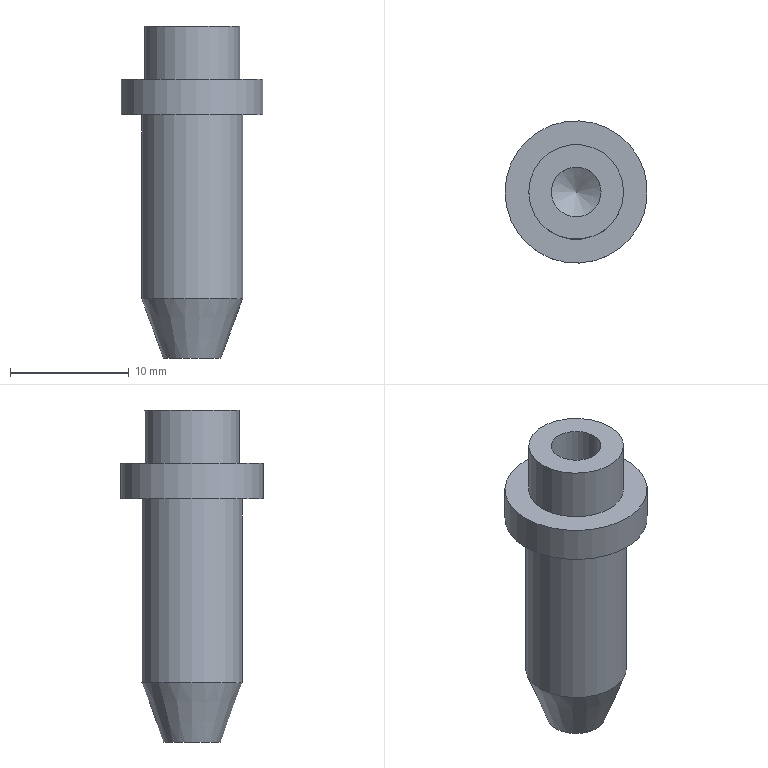Part | NX | features BREP 1 | 1 solid | 10 faces | box 12 x 12 x 28 mm | volume 1447 mm3 | plane 4 | cylinder 4 | cone 2 | commonest cylinder face diameters 4.2 x1 8 x1 8.5 x1 12 x1
STEP:
#1=CARTESIAN_POINT('',(2.1,0.,0.));
#2=VERTEX_POINT('',#1);
#3=CARTESIAN_POINT('',(0.,0.,0.));
#4=DIRECTION('',(0.,0.,1.));
#5=DIRECTION('',(1.,0.,0.));
#6=AXIS2_PLACEMENT_3D('',#3,#4,#5);
#7=CIRCLE('',#6,2.1);
#8=EDGE_CURVE('',#2,#2,#7,.T.);
#9=ORIENTED_EDGE('',*,*,#8,.F.);
#10=EDGE_LOOP('',(#9));
#11=FACE_BOUND('',#10,.T.);
#12=CARTESIAN_POINT('',(-4.,0.,0.));
#13=VERTEX_POINT('',#12);
#14=CARTESIAN_POINT('',(0.,0.,0.));
#15=DIRECTION('',(0.,0.,-1.));
#16=DIRECTION('',(-1.,0.,0.));
#17=AXIS2_PLACEMENT_3D('',#14,#15,#16);
#18=CIRCLE('',#17,4.);
#19=EDGE_CURVE('',#13,#13,#18,.T.);
#20=ORIENTED_EDGE('',*,*,#19,.F.);
#21=EDGE_LOOP('',(#20));
#22=FACE_BOUND('',#21,.T.);
#23=CARTESIAN_POINT('',(0.,0.,0.));
#24=DIRECTION('',(0.,0.,-1.));
#25=DIRECTION('',(1.,0.,0.));
#26=AXIS2_PLACEMENT_3D('',#23,#24,#25);
#27=PLANE('',#26);
#28=ADVANCED_FACE('',(#11,#22),#27,.F.);
#29=CARTESIAN_POINT('',(-4.,0.,-4.5));
#30=VERTEX_POINT('',#29);
#31=CARTESIAN_POINT('',(0.,0.,-4.5));
#32=DIRECTION('',(0.,0.,-1.));
#33=DIRECTION('',(-1.,0.,0.));
#34=AXIS2_PLACEMENT_3D('',#31,#32,#33);
#35=CIRCLE('',#34,4.);
#36=EDGE_CURVE('',#30,#30,#35,.T.);
#37=ORIENTED_EDGE('',*,*,#36,.F.);
#38=EDGE_LOOP('',(#37));
#39=FACE_BOUND('',#38,.T.);
#40=ORIENTED_EDGE('',*,*,#19,.T.);
#41=EDGE_LOOP('',(#40));
#42=FACE_BOUND('',#41,.T.);
#43=CARTESIAN_POINT('',(0.,0.,0.));
#44=DIRECTION('',(0.,0.,-1.));
#45=DIRECTION('',(1.,0.,0.));
#46=AXIS2_PLACEMENT_3D('',#43,#44,#45);
#47=CYLINDRICAL_SURFACE('',#46,4.);
#48=ADVANCED_FACE('',(#39,#42),#47,.T.);
#49=CARTESIAN_POINT('',(-6.,0.,-4.5));
#50=VERTEX_POINT('',#49);
#51=CARTESIAN_POINT('',(0.,0.,-4.5));
#52=DIRECTION('',(0.,0.,-1.));
#53=DIRECTION('',(-1.,0.,0.));
#54=AXIS2_PLACEMENT_3D('',#51,#52,#53);
#55=CIRCLE('',#54,6.);
#56=EDGE_CURVE('',#50,#50,#55,.T.);
#57=ORIENTED_EDGE('',*,*,#56,.F.);
#58=EDGE_LOOP('',(#57));
#59=FACE_BOUND('',#58,.T.);
#60=ORIENTED_EDGE('',*,*,#36,.T.);
#61=EDGE_LOOP('',(#60));
#62=FACE_BOUND('',#61,.T.);
#63=CARTESIAN_POINT('',(4.,0.,-4.5));
#64=DIRECTION('',(0.,0.,-1.));
#65=DIRECTION('',(1.,0.,0.));
#66=AXIS2_PLACEMENT_3D('',#63,#64,#65);
#67=PLANE('',#66);
#68=ADVANCED_FACE('',(#59,#62),#67,.F.);
#69=CARTESIAN_POINT('',(-6.,0.,-7.5));
#70=VERTEX_POINT('',#69);
#71=CARTESIAN_POINT('',(0.,0.,-7.5));
#72=DIRECTION('',(0.,0.,-1.));
#73=DIRECTION('',(-1.,0.,0.));
#74=AXIS2_PLACEMENT_3D('',#71,#72,#73);
#75=CIRCLE('',#74,6.);
#76=EDGE_CURVE('',#70,#70,#75,.T.);
#77=ORIENTED_EDGE('',*,*,#76,.F.);
#78=EDGE_LOOP('',(#77));
#79=FACE_BOUND('',#78,.T.);
#80=ORIENTED_EDGE('',*,*,#56,.T.);
#81=EDGE_LOOP('',(#80));
#82=FACE_BOUND('',#81,.T.);
#83=CARTESIAN_POINT('',(0.,0.,0.));
#84=DIRECTION('',(0.,0.,-1.));
#85=DIRECTION('',(1.,0.,0.));
#86=AXIS2_PLACEMENT_3D('',#83,#84,#85);
#87=CYLINDRICAL_SURFACE('',#86,6.);
#88=ADVANCED_FACE('',(#79,#82),#87,.T.);
#89=CARTESIAN_POINT('',(-4.25,0.,-7.5));
#90=VERTEX_POINT('',#89);
#91=CARTESIAN_POINT('',(0.,0.,-7.5));
#92=DIRECTION('',(0.,0.,-1.));
#93=DIRECTION('',(-1.,0.,0.));
#94=AXIS2_PLACEMENT_3D('',#91,#92,#93);
#95=CIRCLE('',#94,4.25);
#96=EDGE_CURVE('',#90,#90,#95,.T.);
#97=ORIENTED_EDGE('',*,*,#96,.F.);
#98=EDGE_LOOP('',(#97));
#99=FACE_BOUND('',#98,.T.);
#100=ORIENTED_EDGE('',*,*,#76,.T.);
#101=EDGE_LOOP('',(#100));
#102=FACE_BOUND('',#101,.T.);
#103=CARTESIAN_POINT('',(6.,0.,-7.5));
#104=DIRECTION('',(0.,0.,1.));
#105=DIRECTION('',(-1.,0.,0.));
#106=AXIS2_PLACEMENT_3D('',#103,#104,#105);
#107=PLANE('',#106);
#108=ADVANCED_FACE('',(#99,#102),#107,.F.);
#109=CARTESIAN_POINT('',(-4.25,0.,-23.));
#110=VERTEX_POINT('',#109);
#111=CARTESIAN_POINT('',(0.,0.,-23.));
#112=DIRECTION('',(0.,0.,-1.));
#113=DIRECTION('',(-1.,0.,0.));
#114=AXIS2_PLACEMENT_3D('',#111,#112,#113);
#115=CIRCLE('',#114,4.25);
#116=EDGE_CURVE('',#110,#110,#115,.T.);
#117=ORIENTED_EDGE('',*,*,#116,.F.);
#118=EDGE_LOOP('',(#117));
#119=FACE_BOUND('',#118,.T.);
#120=ORIENTED_EDGE('',*,*,#96,.T.);
#121=EDGE_LOOP('',(#120));
#122=FACE_BOUND('',#121,.T.);
#123=CARTESIAN_POINT('',(0.,0.,0.));
#124=DIRECTION('',(0.,0.,-1.));
#125=DIRECTION('',(1.,0.,0.));
#126=AXIS2_PLACEMENT_3D('',#123,#124,#125);
#127=CYLINDRICAL_SURFACE('',#126,4.25);
#128=ADVANCED_FACE('',(#119,#122),#127,.T.);
#129=CARTESIAN_POINT('',(-2.43,0.,-28.));
#130=VERTEX_POINT('',#129);
#131=CARTESIAN_POINT('',(0.,0.,-28.));
#132=DIRECTION('',(0.,0.,-1.));
#133=DIRECTION('',(-1.,0.,0.));
#134=AXIS2_PLACEMENT_3D('',#131,#132,#133);
#135=CIRCLE('',#134,2.43);
#136=EDGE_CURVE('',#130,#130,#135,.T.);
#137=ORIENTED_EDGE('',*,*,#136,.F.);
#138=EDGE_LOOP('',(#137));
#139=FACE_BOUND('',#138,.T.);
#140=ORIENTED_EDGE('',*,*,#116,.T.);
#141=EDGE_LOOP('',(#140));
#142=FACE_BOUND('',#141,.T.);
#143=CARTESIAN_POINT('',(0.,0.,-23.));
#144=DIRECTION('',(0.,0.,1.));
#145=DIRECTION('',(-1.,0.,0.));
#146=AXIS2_PLACEMENT_3D('',#143,#144,#145);
#147=CONICAL_SURFACE('',#146,4.25,0.3491);
#148=ADVANCED_FACE('',(#139,#142),#147,.T.);
#149=ORIENTED_EDGE('',*,*,#136,.T.);
#150=EDGE_LOOP('',(#149));
#151=FACE_BOUND('',#150,.T.);
#152=CARTESIAN_POINT('',(2.43,0.,-28.));
#153=DIRECTION('',(0.,0.,1.));
#154=DIRECTION('',(-1.,0.,0.));
#155=AXIS2_PLACEMENT_3D('',#152,#153,#154);
#156=PLANE('',#155);
#157=ADVANCED_FACE('',(#151),#156,.F.);
#158=CARTESIAN_POINT('',(0.,0.,-13.662));
#159=VERTEX_POINT('',#158);
#160=VERTEX_LOOP('',#159);
#161=FACE_BOUND('',#160,.T.);
#162=CARTESIAN_POINT('',(2.1,0.,-12.4));
#163=VERTEX_POINT('',#162);
#164=CARTESIAN_POINT('',(0.,0.,-12.4));
#165=DIRECTION('',(0.,0.,1.));
#166=DIRECTION('',(1.,0.,0.));
#167=AXIS2_PLACEMENT_3D('',#164,#165,#166);
#168=CIRCLE('',#167,2.1);
#169=EDGE_CURVE('',#163,#163,#168,.T.);
#170=ORIENTED_EDGE('',*,*,#169,.T.);
#171=EDGE_LOOP('',(#170));
#172=FACE_BOUND('',#171,.T.);
#173=CARTESIAN_POINT('',(0.,0.,-12.4));
#174=DIRECTION('',(0.,0.,1.));
#175=DIRECTION('',(-1.,0.,0.));
#176=AXIS2_PLACEMENT_3D('',#173,#174,#175);
#177=CONICAL_SURFACE('',#176,2.1,1.03);
#178=ADVANCED_FACE('',(#161,#172),#177,.F.);
#179=ORIENTED_EDGE('',*,*,#169,.F.);
#180=EDGE_LOOP('',(#179));
#181=FACE_BOUND('',#180,.T.);
#182=ORIENTED_EDGE('',*,*,#8,.T.);
#183=EDGE_LOOP('',(#182));
#184=FACE_BOUND('',#183,.T.);
#185=CARTESIAN_POINT('',(0.,0.,0.));
#186=DIRECTION('',(0.,0.,1.));
#187=DIRECTION('',(-1.,0.,0.));
#188=AXIS2_PLACEMENT_3D('',#185,#186,#187);
#189=CYLINDRICAL_SURFACE('',#188,2.1);
#190=ADVANCED_FACE('',(#181,#184),#189,.F.);
#191=CLOSED_SHELL('',(#28,#48,#68,#88,#108,#128,#148,#157,#178,#190));
#192=MANIFOLD_SOLID_BREP('',#191);
#193=(LENGTH_UNIT()NAMED_UNIT(*)SI_UNIT(.MILLI.,.METRE.));
#194=UNCERTAINTY_MEASURE_WITH_UNIT(LENGTH_MEASURE(0.00001),#193,'','');
#195=(NAMED_UNIT(*)PLANE_ANGLE_UNIT()SI_UNIT($,.RADIAN.));
#196=(NAMED_UNIT(*)SI_UNIT($,.STERADIAN.)SOLID_ANGLE_UNIT());
#197=(GEOMETRIC_REPRESENTATION_CONTEXT(3)GLOBAL_UNCERTAINTY_ASSIGNED_CONTEXT((#194))GLOBAL_UNIT_ASSIGNED_CONTEXT((#193,#195,#196))REPRESENTATION_CONTEXT('',''));
#198=ADVANCED_BREP_SHAPE_REPRESENTATION('',(#192),#197);